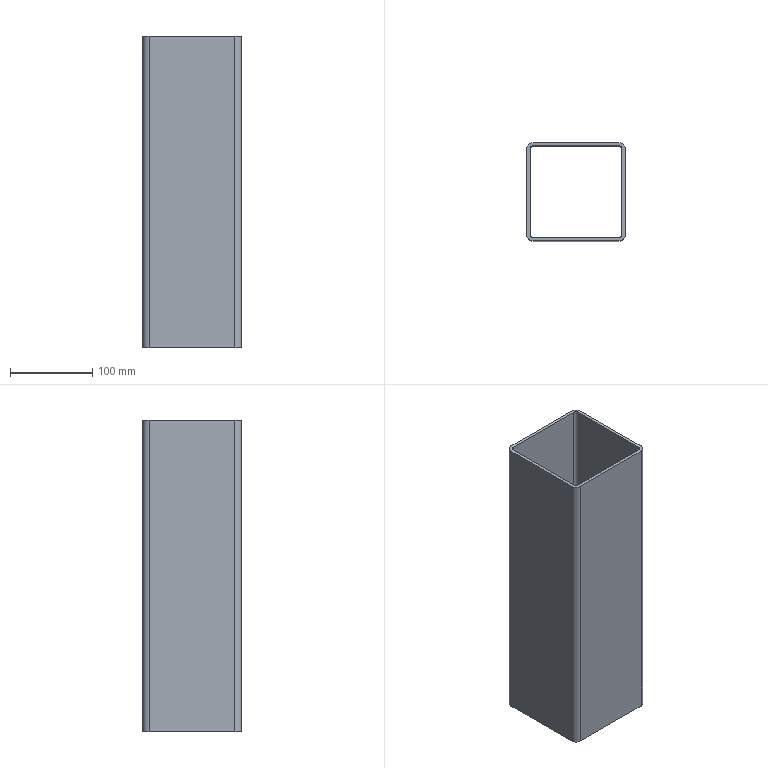Part | SolidWorks | features ICE 1, LibraryFeature 1 | 1 solid | 18 faces | box 120 x 120 x 380 mm | volume 689623 mm3 | plane 10 | cylinder 8 | commonest cylinder face diameters 8 x4 16 x4
STEP:
#1=CARTESIAN_POINT('',(52.,60.,-190.));
#2=VERTEX_POINT('',#1);
#3=CARTESIAN_POINT('',(-52.,60.,-190.));
#4=VERTEX_POINT('',#3);
#5=CARTESIAN_POINT('',(0.,60.,-190.));
#6=DIRECTION('',(-1.,0.,0.));
#7=VECTOR('',#6,1000.);
#8=LINE('',#5,#7);
#9=EDGE_CURVE('',#2,#4,#8,.T.);
#10=ORIENTED_EDGE('',*,*,#9,.T.);
#11=CARTESIAN_POINT('',(-52.,60.,190.));
#12=VERTEX_POINT('',#11);
#13=CARTESIAN_POINT('',(-52.,60.,190.));
#14=DIRECTION('',(0.,0.,-1.));
#15=VECTOR('',#14,1000.);
#16=LINE('',#13,#15);
#17=EDGE_CURVE('',#12,#4,#16,.T.);
#18=ORIENTED_EDGE('',*,*,#17,.F.);
#19=CARTESIAN_POINT('',(52.,60.,190.));
#20=VERTEX_POINT('',#19);
#21=CARTESIAN_POINT('',(0.,60.,190.));
#22=DIRECTION('',(-1.,0.,0.));
#23=VECTOR('',#22,1000.);
#24=LINE('',#21,#23);
#25=EDGE_CURVE('',#20,#12,#24,.T.);
#26=ORIENTED_EDGE('',*,*,#25,.F.);
#27=CARTESIAN_POINT('',(52.,60.,190.));
#28=DIRECTION('',(0.,0.,-1.));
#29=VECTOR('',#28,1000.);
#30=LINE('',#27,#29);
#31=EDGE_CURVE('',#20,#2,#30,.T.);
#32=ORIENTED_EDGE('',*,*,#31,.T.);
#33=EDGE_LOOP('',(#10,#18,#26,#32));
#34=FACE_OUTER_BOUND('',#33,.T.);
#35=CARTESIAN_POINT('',(0.,60.,190.));
#36=DIRECTION('',(0.,-1.,0.));
#37=DIRECTION('',(0.,0.,-1.));
#38=AXIS2_PLACEMENT_3D('',#35,#36,#37);
#39=PLANE('',#38);
#40=ADVANCED_FACE('',(#34),#39,.F.);
#41=CARTESIAN_POINT('',(-60.,52.,-190.));
#42=VERTEX_POINT('',#41);
#43=CARTESIAN_POINT('',(-52.,52.,-190.));
#44=DIRECTION('',(0.,0.,1.));
#45=DIRECTION('',(1.,0.,0.));
#46=AXIS2_PLACEMENT_3D('',#43,#44,#45);
#47=CIRCLE('',#46,8.);
#48=EDGE_CURVE('',#4,#42,#47,.T.);
#49=ORIENTED_EDGE('',*,*,#48,.T.);
#50=CARTESIAN_POINT('',(-60.,52.,190.));
#51=VERTEX_POINT('',#50);
#52=CARTESIAN_POINT('',(-60.,52.,190.));
#53=DIRECTION('',(0.,0.,-1.));
#54=VECTOR('',#53,1000.);
#55=LINE('',#52,#54);
#56=EDGE_CURVE('',#51,#42,#55,.T.);
#57=ORIENTED_EDGE('',*,*,#56,.F.);
#58=CARTESIAN_POINT('',(-52.,52.,190.));
#59=DIRECTION('',(0.,0.,1.));
#60=DIRECTION('',(1.,0.,0.));
#61=AXIS2_PLACEMENT_3D('',#58,#59,#60);
#62=CIRCLE('',#61,8.);
#63=EDGE_CURVE('',#12,#51,#62,.T.);
#64=ORIENTED_EDGE('',*,*,#63,.F.);
#65=ORIENTED_EDGE('',*,*,#17,.T.);
#66=EDGE_LOOP('',(#49,#57,#64,#65));
#67=FACE_OUTER_BOUND('',#66,.T.);
#68=CARTESIAN_POINT('',(-52.,52.,190.));
#69=DIRECTION('',(0.,0.,-1.));
#70=DIRECTION('',(-1.,0.,0.));
#71=AXIS2_PLACEMENT_3D('',#68,#69,#70);
#72=CYLINDRICAL_SURFACE('',#71,8.);
#73=ADVANCED_FACE('',(#67),#72,.T.);
#74=CARTESIAN_POINT('',(-60.,-52.,-190.));
#75=VERTEX_POINT('',#74);
#76=CARTESIAN_POINT('',(-60.,0.,-190.));
#77=DIRECTION('',(0.,1.,0.));
#78=VECTOR('',#77,1000.);
#79=LINE('',#76,#78);
#80=EDGE_CURVE('',#75,#42,#79,.T.);
#81=ORIENTED_EDGE('',*,*,#80,.F.);
#82=CARTESIAN_POINT('',(-60.,-52.,190.));
#83=VERTEX_POINT('',#82);
#84=CARTESIAN_POINT('',(-60.,-52.,190.));
#85=DIRECTION('',(0.,0.,-1.));
#86=VECTOR('',#85,1000.);
#87=LINE('',#84,#86);
#88=EDGE_CURVE('',#83,#75,#87,.T.);
#89=ORIENTED_EDGE('',*,*,#88,.F.);
#90=CARTESIAN_POINT('',(-60.,0.,190.));
#91=DIRECTION('',(0.,1.,0.));
#92=VECTOR('',#91,1000.);
#93=LINE('',#90,#92);
#94=EDGE_CURVE('',#83,#51,#93,.T.);
#95=ORIENTED_EDGE('',*,*,#94,.T.);
#96=ORIENTED_EDGE('',*,*,#56,.T.);
#97=EDGE_LOOP('',(#81,#89,#95,#96));
#98=FACE_OUTER_BOUND('',#97,.T.);
#99=CARTESIAN_POINT('',(-60.,0.,190.));
#100=DIRECTION('',(-1.,0.,0.));
#101=DIRECTION('',(0.,0.,1.));
#102=AXIS2_PLACEMENT_3D('',#99,#100,#101);
#103=PLANE('',#102);
#104=ADVANCED_FACE('',(#98),#103,.T.);
#105=CARTESIAN_POINT('',(-52.,-60.,-190.));
#106=VERTEX_POINT('',#105);
#107=CARTESIAN_POINT('',(-52.,-52.,-190.));
#108=DIRECTION('',(0.,0.,1.));
#109=DIRECTION('',(1.,0.,0.));
#110=AXIS2_PLACEMENT_3D('',#107,#108,#109);
#111=CIRCLE('',#110,8.);
#112=EDGE_CURVE('',#75,#106,#111,.T.);
#113=ORIENTED_EDGE('',*,*,#112,.T.);
#114=CARTESIAN_POINT('',(-52.,-60.,190.));
#115=VERTEX_POINT('',#114);
#116=CARTESIAN_POINT('',(-52.,-60.,190.));
#117=DIRECTION('',(0.,0.,-1.));
#118=VECTOR('',#117,1000.);
#119=LINE('',#116,#118);
#120=EDGE_CURVE('',#115,#106,#119,.T.);
#121=ORIENTED_EDGE('',*,*,#120,.F.);
#122=CARTESIAN_POINT('',(-52.,-52.,190.));
#123=DIRECTION('',(0.,0.,1.));
#124=DIRECTION('',(1.,0.,0.));
#125=AXIS2_PLACEMENT_3D('',#122,#123,#124);
#126=CIRCLE('',#125,8.);
#127=EDGE_CURVE('',#83,#115,#126,.T.);
#128=ORIENTED_EDGE('',*,*,#127,.F.);
#129=ORIENTED_EDGE('',*,*,#88,.T.);
#130=EDGE_LOOP('',(#113,#121,#128,#129));
#131=FACE_OUTER_BOUND('',#130,.T.);
#132=CARTESIAN_POINT('',(-52.,-52.,190.));
#133=DIRECTION('',(0.,0.,-1.));
#134=DIRECTION('',(-1.,0.,0.));
#135=AXIS2_PLACEMENT_3D('',#132,#133,#134);
#136=CYLINDRICAL_SURFACE('',#135,8.);
#137=ADVANCED_FACE('',(#131),#136,.T.);
#138=CARTESIAN_POINT('',(52.,-60.,-190.));
#139=VERTEX_POINT('',#138);
#140=CARTESIAN_POINT('',(0.,-60.,-190.));
#141=DIRECTION('',(1.,0.,0.));
#142=VECTOR('',#141,1000.);
#143=LINE('',#140,#142);
#144=EDGE_CURVE('',#106,#139,#143,.T.);
#145=ORIENTED_EDGE('',*,*,#144,.T.);
#146=CARTESIAN_POINT('',(52.,-60.,190.));
#147=VERTEX_POINT('',#146);
#148=CARTESIAN_POINT('',(52.,-60.,190.));
#149=DIRECTION('',(0.,0.,-1.));
#150=VECTOR('',#149,1000.);
#151=LINE('',#148,#150);
#152=EDGE_CURVE('',#147,#139,#151,.T.);
#153=ORIENTED_EDGE('',*,*,#152,.F.);
#154=CARTESIAN_POINT('',(0.,-60.,190.));
#155=DIRECTION('',(1.,0.,0.));
#156=VECTOR('',#155,1000.);
#157=LINE('',#154,#156);
#158=EDGE_CURVE('',#115,#147,#157,.T.);
#159=ORIENTED_EDGE('',*,*,#158,.F.);
#160=ORIENTED_EDGE('',*,*,#120,.T.);
#161=EDGE_LOOP('',(#145,#153,#159,#160));
#162=FACE_OUTER_BOUND('',#161,.T.);
#163=CARTESIAN_POINT('',(0.,-60.,190.));
#164=DIRECTION('',(0.,1.,0.));
#165=DIRECTION('',(0.,0.,1.));
#166=AXIS2_PLACEMENT_3D('',#163,#164,#165);
#167=PLANE('',#166);
#168=ADVANCED_FACE('',(#162),#167,.F.);
#169=CARTESIAN_POINT('',(60.,-52.,-190.));
#170=VERTEX_POINT('',#169);
#171=CARTESIAN_POINT('',(52.,-52.,-190.));
#172=DIRECTION('',(0.,0.,1.));
#173=DIRECTION('',(1.,0.,0.));
#174=AXIS2_PLACEMENT_3D('',#171,#172,#173);
#175=CIRCLE('',#174,8.);
#176=EDGE_CURVE('',#139,#170,#175,.T.);
#177=ORIENTED_EDGE('',*,*,#176,.T.);
#178=CARTESIAN_POINT('',(60.,-52.,190.));
#179=VERTEX_POINT('',#178);
#180=CARTESIAN_POINT('',(60.,-52.,190.));
#181=DIRECTION('',(0.,0.,-1.));
#182=VECTOR('',#181,1000.);
#183=LINE('',#180,#182);
#184=EDGE_CURVE('',#179,#170,#183,.T.);
#185=ORIENTED_EDGE('',*,*,#184,.F.);
#186=CARTESIAN_POINT('',(52.,-52.,190.));
#187=DIRECTION('',(0.,0.,1.));
#188=DIRECTION('',(1.,0.,0.));
#189=AXIS2_PLACEMENT_3D('',#186,#187,#188);
#190=CIRCLE('',#189,8.);
#191=EDGE_CURVE('',#147,#179,#190,.T.);
#192=ORIENTED_EDGE('',*,*,#191,.F.);
#193=ORIENTED_EDGE('',*,*,#152,.T.);
#194=EDGE_LOOP('',(#177,#185,#192,#193));
#195=FACE_OUTER_BOUND('',#194,.T.);
#196=CARTESIAN_POINT('',(52.,-52.,190.));
#197=DIRECTION('',(0.,0.,-1.));
#198=DIRECTION('',(-1.,0.,0.));
#199=AXIS2_PLACEMENT_3D('',#196,#197,#198);
#200=CYLINDRICAL_SURFACE('',#199,8.);
#201=ADVANCED_FACE('',(#195),#200,.T.);
#202=CARTESIAN_POINT('',(60.,52.,-190.));
#203=VERTEX_POINT('',#202);
#204=CARTESIAN_POINT('',(60.,0.,-190.));
#205=DIRECTION('',(0.,-1.,0.));
#206=VECTOR('',#205,1000.);
#207=LINE('',#204,#206);
#208=EDGE_CURVE('',#203,#170,#207,.T.);
#209=ORIENTED_EDGE('',*,*,#208,.F.);
#210=CARTESIAN_POINT('',(60.,52.,190.));
#211=VERTEX_POINT('',#210);
#212=CARTESIAN_POINT('',(60.,52.,190.));
#213=DIRECTION('',(0.,0.,-1.));
#214=VECTOR('',#213,1000.);
#215=LINE('',#212,#214);
#216=EDGE_CURVE('',#211,#203,#215,.T.);
#217=ORIENTED_EDGE('',*,*,#216,.F.);
#218=CARTESIAN_POINT('',(60.,0.,190.));
#219=DIRECTION('',(0.,-1.,0.));
#220=VECTOR('',#219,1000.);
#221=LINE('',#218,#220);
#222=EDGE_CURVE('',#211,#179,#221,.T.);
#223=ORIENTED_EDGE('',*,*,#222,.T.);
#224=ORIENTED_EDGE('',*,*,#184,.T.);
#225=EDGE_LOOP('',(#209,#217,#223,#224));
#226=FACE_OUTER_BOUND('',#225,.T.);
#227=CARTESIAN_POINT('',(60.,0.,190.));
#228=DIRECTION('',(1.,0.,0.));
#229=DIRECTION('',(0.,0.,-1.));
#230=AXIS2_PLACEMENT_3D('',#227,#228,#229);
#231=PLANE('',#230);
#232=ADVANCED_FACE('',(#226),#231,.T.);
#233=CARTESIAN_POINT('',(-56.,-52.,-190.));
#234=VERTEX_POINT('',#233);
#235=CARTESIAN_POINT('',(-52.,-56.,-190.));
#236=VERTEX_POINT('',#235);
#237=CARTESIAN_POINT('',(-52.,-52.,-190.));
#238=DIRECTION('',(0.,0.,1.));
#239=DIRECTION('',(1.,0.,0.));
#240=AXIS2_PLACEMENT_3D('',#237,#238,#239);
#241=CIRCLE('',#240,4.);
#242=EDGE_CURVE('',#234,#236,#241,.T.);
#243=ORIENTED_EDGE('',*,*,#242,.F.);
#244=CARTESIAN_POINT('',(-56.,-52.,190.));
#245=VERTEX_POINT('',#244);
#246=CARTESIAN_POINT('',(-56.,-52.,190.));
#247=DIRECTION('',(0.,0.,-1.));
#248=VECTOR('',#247,1000.);
#249=LINE('',#246,#248);
#250=EDGE_CURVE('',#245,#234,#249,.T.);
#251=ORIENTED_EDGE('',*,*,#250,.F.);
#252=CARTESIAN_POINT('',(-52.,-56.,190.));
#253=VERTEX_POINT('',#252);
#254=CARTESIAN_POINT('',(-52.,-52.,190.));
#255=DIRECTION('',(0.,0.,1.));
#256=DIRECTION('',(1.,0.,0.));
#257=AXIS2_PLACEMENT_3D('',#254,#255,#256);
#258=CIRCLE('',#257,4.);
#259=EDGE_CURVE('',#245,#253,#258,.T.);
#260=ORIENTED_EDGE('',*,*,#259,.T.);
#261=CARTESIAN_POINT('',(-52.,-56.,190.));
#262=DIRECTION('',(0.,0.,-1.));
#263=VECTOR('',#262,1000.);
#264=LINE('',#261,#263);
#265=EDGE_CURVE('',#253,#236,#264,.T.);
#266=ORIENTED_EDGE('',*,*,#265,.T.);
#267=EDGE_LOOP('',(#243,#251,#260,#266));
#268=FACE_OUTER_BOUND('',#267,.T.);
#269=CARTESIAN_POINT('',(-52.,-52.,190.));
#270=DIRECTION('',(0.,0.,-1.));
#271=DIRECTION('',(-1.,0.,0.));
#272=AXIS2_PLACEMENT_3D('',#269,#270,#271);
#273=CYLINDRICAL_SURFACE('',#272,4.);
#274=ADVANCED_FACE('',(#268),#273,.F.);
#275=CARTESIAN_POINT('',(-56.,52.,-190.));
#276=VERTEX_POINT('',#275);
#277=CARTESIAN_POINT('',(-56.,0.,-190.));
#278=DIRECTION('',(0.,1.,0.));
#279=VECTOR('',#278,1000.);
#280=LINE('',#277,#279);
#281=EDGE_CURVE('',#234,#276,#280,.T.);
#282=ORIENTED_EDGE('',*,*,#281,.T.);
#283=CARTESIAN_POINT('',(-56.,52.,190.));
#284=VERTEX_POINT('',#283);
#285=CARTESIAN_POINT('',(-56.,52.,190.));
#286=DIRECTION('',(0.,0.,-1.));
#287=VECTOR('',#286,1000.);
#288=LINE('',#285,#287);
#289=EDGE_CURVE('',#284,#276,#288,.T.);
#290=ORIENTED_EDGE('',*,*,#289,.F.);
#291=CARTESIAN_POINT('',(-56.,0.,190.));
#292=DIRECTION('',(0.,1.,0.));
#293=VECTOR('',#292,1000.);
#294=LINE('',#291,#293);
#295=EDGE_CURVE('',#245,#284,#294,.T.);
#296=ORIENTED_EDGE('',*,*,#295,.F.);
#297=ORIENTED_EDGE('',*,*,#250,.T.);
#298=EDGE_LOOP('',(#282,#290,#296,#297));
#299=FACE_OUTER_BOUND('',#298,.T.);
#300=CARTESIAN_POINT('',(-56.,0.,190.));
#301=DIRECTION('',(-1.,0.,0.));
#302=DIRECTION('',(0.,0.,1.));
#303=AXIS2_PLACEMENT_3D('',#300,#301,#302);
#304=PLANE('',#303);
#305=ADVANCED_FACE('',(#299),#304,.F.);
#306=CARTESIAN_POINT('',(-52.,56.,-190.));
#307=VERTEX_POINT('',#306);
#308=CARTESIAN_POINT('',(-52.,52.,-190.));
#309=DIRECTION('',(0.,0.,1.));
#310=DIRECTION('',(1.,0.,0.));
#311=AXIS2_PLACEMENT_3D('',#308,#309,#310);
#312=CIRCLE('',#311,4.);
#313=EDGE_CURVE('',#307,#276,#312,.T.);
#314=ORIENTED_EDGE('',*,*,#313,.F.);
#315=CARTESIAN_POINT('',(-52.,56.,190.));
#316=VERTEX_POINT('',#315);
#317=CARTESIAN_POINT('',(-52.,56.,190.));
#318=DIRECTION('',(0.,0.,-1.));
#319=VECTOR('',#318,1000.);
#320=LINE('',#317,#319);
#321=EDGE_CURVE('',#316,#307,#320,.T.);
#322=ORIENTED_EDGE('',*,*,#321,.F.);
#323=CARTESIAN_POINT('',(-52.,52.,190.));
#324=DIRECTION('',(0.,0.,1.));
#325=DIRECTION('',(1.,0.,0.));
#326=AXIS2_PLACEMENT_3D('',#323,#324,#325);
#327=CIRCLE('',#326,4.);
#328=EDGE_CURVE('',#316,#284,#327,.T.);
#329=ORIENTED_EDGE('',*,*,#328,.T.);
#330=ORIENTED_EDGE('',*,*,#289,.T.);
#331=EDGE_LOOP('',(#314,#322,#329,#330));
#332=FACE_OUTER_BOUND('',#331,.T.);
#333=CARTESIAN_POINT('',(-52.,52.,190.));
#334=DIRECTION('',(0.,0.,-1.));
#335=DIRECTION('',(-1.,0.,0.));
#336=AXIS2_PLACEMENT_3D('',#333,#334,#335);
#337=CYLINDRICAL_SURFACE('',#336,4.);
#338=ADVANCED_FACE('',(#332),#337,.F.);
#339=CARTESIAN_POINT('',(52.,56.,-190.));
#340=VERTEX_POINT('',#339);
#341=CARTESIAN_POINT('',(0.,56.,-190.));
#342=DIRECTION('',(-1.,0.,0.));
#343=VECTOR('',#342,1000.);
#344=LINE('',#341,#343);
#345=EDGE_CURVE('',#340,#307,#344,.T.);
#346=ORIENTED_EDGE('',*,*,#345,.F.);
#347=CARTESIAN_POINT('',(52.,56.,190.));
#348=VERTEX_POINT('',#347);
#349=CARTESIAN_POINT('',(52.,56.,190.));
#350=DIRECTION('',(0.,0.,-1.));
#351=VECTOR('',#350,1000.);
#352=LINE('',#349,#351);
#353=EDGE_CURVE('',#348,#340,#352,.T.);
#354=ORIENTED_EDGE('',*,*,#353,.F.);
#355=CARTESIAN_POINT('',(0.,56.,190.));
#356=DIRECTION('',(-1.,0.,0.));
#357=VECTOR('',#356,1000.);
#358=LINE('',#355,#357);
#359=EDGE_CURVE('',#348,#316,#358,.T.);
#360=ORIENTED_EDGE('',*,*,#359,.T.);
#361=ORIENTED_EDGE('',*,*,#321,.T.);
#362=EDGE_LOOP('',(#346,#354,#360,#361));
#363=FACE_OUTER_BOUND('',#362,.T.);
#364=CARTESIAN_POINT('',(0.,56.,190.));
#365=DIRECTION('',(0.,-1.,0.));
#366=DIRECTION('',(0.,0.,-1.));
#367=AXIS2_PLACEMENT_3D('',#364,#365,#366);
#368=PLANE('',#367);
#369=ADVANCED_FACE('',(#363),#368,.T.);
#370=CARTESIAN_POINT('',(56.,52.,-190.));
#371=VERTEX_POINT('',#370);
#372=CARTESIAN_POINT('',(52.,52.,-190.));
#373=DIRECTION('',(0.,0.,1.));
#374=DIRECTION('',(1.,0.,0.));
#375=AXIS2_PLACEMENT_3D('',#372,#373,#374);
#376=CIRCLE('',#375,4.);
#377=EDGE_CURVE('',#371,#340,#376,.T.);
#378=ORIENTED_EDGE('',*,*,#377,.F.);
#379=CARTESIAN_POINT('',(56.,52.,190.));
#380=VERTEX_POINT('',#379);
#381=CARTESIAN_POINT('',(56.,52.,190.));
#382=DIRECTION('',(0.,0.,-1.));
#383=VECTOR('',#382,1000.);
#384=LINE('',#381,#383);
#385=EDGE_CURVE('',#380,#371,#384,.T.);
#386=ORIENTED_EDGE('',*,*,#385,.F.);
#387=CARTESIAN_POINT('',(52.,52.,190.));
#388=DIRECTION('',(0.,0.,1.));
#389=DIRECTION('',(1.,0.,0.));
#390=AXIS2_PLACEMENT_3D('',#387,#388,#389);
#391=CIRCLE('',#390,4.);
#392=EDGE_CURVE('',#380,#348,#391,.T.);
#393=ORIENTED_EDGE('',*,*,#392,.T.);
#394=ORIENTED_EDGE('',*,*,#353,.T.);
#395=EDGE_LOOP('',(#378,#386,#393,#394));
#396=FACE_OUTER_BOUND('',#395,.T.);
#397=CARTESIAN_POINT('',(52.,52.,190.));
#398=DIRECTION('',(0.,0.,-1.));
#399=DIRECTION('',(-1.,0.,0.));
#400=AXIS2_PLACEMENT_3D('',#397,#398,#399);
#401=CYLINDRICAL_SURFACE('',#400,4.);
#402=ADVANCED_FACE('',(#396),#401,.F.);
#403=CARTESIAN_POINT('',(56.,-52.,-190.));
#404=VERTEX_POINT('',#403);
#405=CARTESIAN_POINT('',(56.,0.,-190.));
#406=DIRECTION('',(0.,-1.,0.));
#407=VECTOR('',#406,1000.);
#408=LINE('',#405,#407);
#409=EDGE_CURVE('',#371,#404,#408,.T.);
#410=ORIENTED_EDGE('',*,*,#409,.T.);
#411=CARTESIAN_POINT('',(56.,-52.,190.));
#412=VERTEX_POINT('',#411);
#413=CARTESIAN_POINT('',(56.,-52.,190.));
#414=DIRECTION('',(0.,0.,-1.));
#415=VECTOR('',#414,1000.);
#416=LINE('',#413,#415);
#417=EDGE_CURVE('',#412,#404,#416,.T.);
#418=ORIENTED_EDGE('',*,*,#417,.F.);
#419=CARTESIAN_POINT('',(56.,0.,190.));
#420=DIRECTION('',(0.,-1.,0.));
#421=VECTOR('',#420,1000.);
#422=LINE('',#419,#421);
#423=EDGE_CURVE('',#380,#412,#422,.T.);
#424=ORIENTED_EDGE('',*,*,#423,.F.);
#425=ORIENTED_EDGE('',*,*,#385,.T.);
#426=EDGE_LOOP('',(#410,#418,#424,#425));
#427=FACE_OUTER_BOUND('',#426,.T.);
#428=CARTESIAN_POINT('',(56.,0.,190.));
#429=DIRECTION('',(1.,0.,0.));
#430=DIRECTION('',(0.,0.,-1.));
#431=AXIS2_PLACEMENT_3D('',#428,#429,#430);
#432=PLANE('',#431);
#433=ADVANCED_FACE('',(#427),#432,.F.);
#434=CARTESIAN_POINT('',(52.,-56.,-190.));
#435=VERTEX_POINT('',#434);
#436=CARTESIAN_POINT('',(52.,-52.,-190.));
#437=DIRECTION('',(0.,0.,1.));
#438=DIRECTION('',(1.,0.,0.));
#439=AXIS2_PLACEMENT_3D('',#436,#437,#438);
#440=CIRCLE('',#439,4.);
#441=EDGE_CURVE('',#435,#404,#440,.T.);
#442=ORIENTED_EDGE('',*,*,#441,.F.);
#443=CARTESIAN_POINT('',(52.,-56.,190.));
#444=VERTEX_POINT('',#443);
#445=CARTESIAN_POINT('',(52.,-56.,190.));
#446=DIRECTION('',(0.,0.,-1.));
#447=VECTOR('',#446,1000.);
#448=LINE('',#445,#447);
#449=EDGE_CURVE('',#444,#435,#448,.T.);
#450=ORIENTED_EDGE('',*,*,#449,.F.);
#451=CARTESIAN_POINT('',(52.,-52.,190.));
#452=DIRECTION('',(0.,0.,1.));
#453=DIRECTION('',(1.,0.,0.));
#454=AXIS2_PLACEMENT_3D('',#451,#452,#453);
#455=CIRCLE('',#454,4.);
#456=EDGE_CURVE('',#444,#412,#455,.T.);
#457=ORIENTED_EDGE('',*,*,#456,.T.);
#458=ORIENTED_EDGE('',*,*,#417,.T.);
#459=EDGE_LOOP('',(#442,#450,#457,#458));
#460=FACE_OUTER_BOUND('',#459,.T.);
#461=CARTESIAN_POINT('',(52.,-52.,190.));
#462=DIRECTION('',(0.,0.,-1.));
#463=DIRECTION('',(-1.,0.,0.));
#464=AXIS2_PLACEMENT_3D('',#461,#462,#463);
#465=CYLINDRICAL_SURFACE('',#464,4.);
#466=ADVANCED_FACE('',(#460),#465,.F.);
#467=CARTESIAN_POINT('',(0.,-56.,-190.));
#468=DIRECTION('',(1.,0.,0.));
#469=VECTOR('',#468,1000.);
#470=LINE('',#467,#469);
#471=EDGE_CURVE('',#236,#435,#470,.T.);
#472=ORIENTED_EDGE('',*,*,#471,.F.);
#473=ORIENTED_EDGE('',*,*,#265,.F.);
#474=CARTESIAN_POINT('',(0.,-56.,190.));
#475=DIRECTION('',(1.,0.,0.));
#476=VECTOR('',#475,1000.);
#477=LINE('',#474,#476);
#478=EDGE_CURVE('',#253,#444,#477,.T.);
#479=ORIENTED_EDGE('',*,*,#478,.T.);
#480=ORIENTED_EDGE('',*,*,#449,.T.);
#481=EDGE_LOOP('',(#472,#473,#479,#480));
#482=FACE_OUTER_BOUND('',#481,.T.);
#483=CARTESIAN_POINT('',(0.,-56.,190.));
#484=DIRECTION('',(0.,1.,0.));
#485=DIRECTION('',(0.,0.,1.));
#486=AXIS2_PLACEMENT_3D('',#483,#484,#485);
#487=PLANE('',#486);
#488=ADVANCED_FACE('',(#482),#487,.T.);
#489=CARTESIAN_POINT('',(52.,52.,-190.));
#490=DIRECTION('',(0.,0.,1.));
#491=DIRECTION('',(1.,0.,0.));
#492=AXIS2_PLACEMENT_3D('',#489,#490,#491);
#493=CIRCLE('',#492,8.);
#494=EDGE_CURVE('',#203,#2,#493,.T.);
#495=ORIENTED_EDGE('',*,*,#494,.T.);
#496=ORIENTED_EDGE('',*,*,#31,.F.);
#497=CARTESIAN_POINT('',(52.,52.,190.));
#498=DIRECTION('',(0.,0.,1.));
#499=DIRECTION('',(1.,0.,0.));
#500=AXIS2_PLACEMENT_3D('',#497,#498,#499);
#501=CIRCLE('',#500,8.);
#502=EDGE_CURVE('',#211,#20,#501,.T.);
#503=ORIENTED_EDGE('',*,*,#502,.F.);
#504=ORIENTED_EDGE('',*,*,#216,.T.);
#505=EDGE_LOOP('',(#495,#496,#503,#504));
#506=FACE_OUTER_BOUND('',#505,.T.);
#507=CARTESIAN_POINT('',(52.,52.,190.));
#508=DIRECTION('',(0.,0.,-1.));
#509=DIRECTION('',(-1.,0.,0.));
#510=AXIS2_PLACEMENT_3D('',#507,#508,#509);
#511=CYLINDRICAL_SURFACE('',#510,8.);
#512=ADVANCED_FACE('',(#506),#511,.T.);
#513=ORIENTED_EDGE('',*,*,#259,.F.);
#514=ORIENTED_EDGE('',*,*,#295,.T.);
#515=ORIENTED_EDGE('',*,*,#328,.F.);
#516=ORIENTED_EDGE('',*,*,#359,.F.);
#517=ORIENTED_EDGE('',*,*,#392,.F.);
#518=ORIENTED_EDGE('',*,*,#423,.T.);
#519=ORIENTED_EDGE('',*,*,#456,.F.);
#520=ORIENTED_EDGE('',*,*,#478,.F.);
#521=EDGE_LOOP('',(#513,#514,#515,#516,#517,#518,#519,#520));
#522=FACE_BOUND('',#521,.T.);
#523=ORIENTED_EDGE('',*,*,#25,.T.);
#524=ORIENTED_EDGE('',*,*,#63,.T.);
#525=ORIENTED_EDGE('',*,*,#94,.F.);
#526=ORIENTED_EDGE('',*,*,#127,.T.);
#527=ORIENTED_EDGE('',*,*,#158,.T.);
#528=ORIENTED_EDGE('',*,*,#191,.T.);
#529=ORIENTED_EDGE('',*,*,#222,.F.);
#530=ORIENTED_EDGE('',*,*,#502,.T.);
#531=EDGE_LOOP('',(#523,#524,#525,#526,#527,#528,#529,#530));
#532=FACE_OUTER_BOUND('',#531,.T.);
#533=CARTESIAN_POINT('',(0.,0.,190.));
#534=DIRECTION('',(0.,0.,1.));
#535=DIRECTION('',(1.,0.,0.));
#536=AXIS2_PLACEMENT_3D('',#533,#534,#535);
#537=PLANE('',#536);
#538=ADVANCED_FACE('',(#522,#532),#537,.T.);
#539=ORIENTED_EDGE('',*,*,#242,.T.);
#540=ORIENTED_EDGE('',*,*,#471,.T.);
#541=ORIENTED_EDGE('',*,*,#441,.T.);
#542=ORIENTED_EDGE('',*,*,#409,.F.);
#543=ORIENTED_EDGE('',*,*,#377,.T.);
#544=ORIENTED_EDGE('',*,*,#345,.T.);
#545=ORIENTED_EDGE('',*,*,#313,.T.);
#546=ORIENTED_EDGE('',*,*,#281,.F.);
#547=EDGE_LOOP('',(#539,#540,#541,#542,#543,#544,#545,#546));
#548=FACE_BOUND('',#547,.T.);
#549=ORIENTED_EDGE('',*,*,#9,.F.);
#550=ORIENTED_EDGE('',*,*,#494,.F.);
#551=ORIENTED_EDGE('',*,*,#208,.T.);
#552=ORIENTED_EDGE('',*,*,#176,.F.);
#553=ORIENTED_EDGE('',*,*,#144,.F.);
#554=ORIENTED_EDGE('',*,*,#112,.F.);
#555=ORIENTED_EDGE('',*,*,#80,.T.);
#556=ORIENTED_EDGE('',*,*,#48,.F.);
#557=EDGE_LOOP('',(#549,#550,#551,#552,#553,#554,#555,#556));
#558=FACE_OUTER_BOUND('',#557,.T.);
#559=CARTESIAN_POINT('',(0.,0.,-190.));
#560=DIRECTION('',(0.,0.,1.));
#561=DIRECTION('',(1.,0.,0.));
#562=AXIS2_PLACEMENT_3D('',#559,#560,#561);
#563=PLANE('',#562);
#564=ADVANCED_FACE('',(#548,#558),#563,.F.);
#565=CLOSED_SHELL('',(#40,#73,#104,#137,#168,#201,#232,#274,#305,#338,#369,#402,#433,#466,#488,#512,#538,#564));
#566=MANIFOLD_SOLID_BREP('',#565);
#567=CARTESIAN_POINT('',(0.,0.,0.));
#568=DIRECTION('',(0.,0.,1.));
#569=DIRECTION('',(1.,0.,0.));
#570=AXIS2_PLACEMENT_3D('',#567,#568,#569);
#571=(LENGTH_UNIT()NAMED_UNIT(*)SI_UNIT(.MILLI.,.METRE.));
#572=UNCERTAINTY_MEASURE_WITH_UNIT(LENGTH_MEASURE(0.00001),#571,'','');
#573=(NAMED_UNIT(*)PLANE_ANGLE_UNIT()SI_UNIT($,.RADIAN.));
#574=(NAMED_UNIT(*)SI_UNIT($,.STERADIAN.)SOLID_ANGLE_UNIT());
#575=(GEOMETRIC_REPRESENTATION_CONTEXT(3)GLOBAL_UNCERTAINTY_ASSIGNED_CONTEXT((#572))GLOBAL_UNIT_ASSIGNED_CONTEXT((#571,#573,#574))REPRESENTATION_CONTEXT('',''));
#576=ADVANCED_BREP_SHAPE_REPRESENTATION('',(#566,#570),#575);